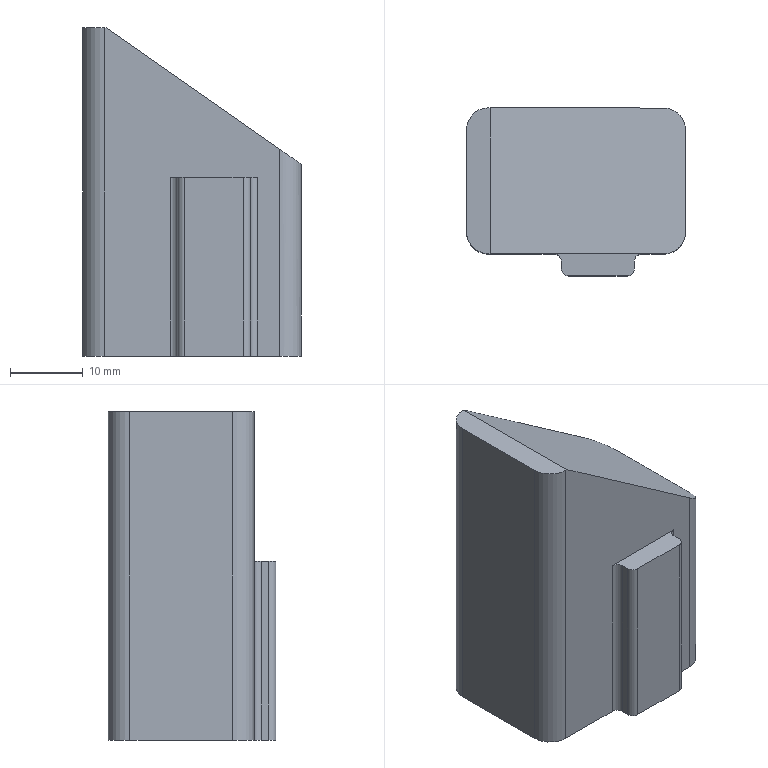Part | STEP file | 1_id858_x_t | 1 solid | 22 faces | box 30 x 23 x 45 mm | volume 21294 mm3 | plane 12 | cylinder 10 | commonest cylinder face diameters 2 x4 6 x4 14.5 x2